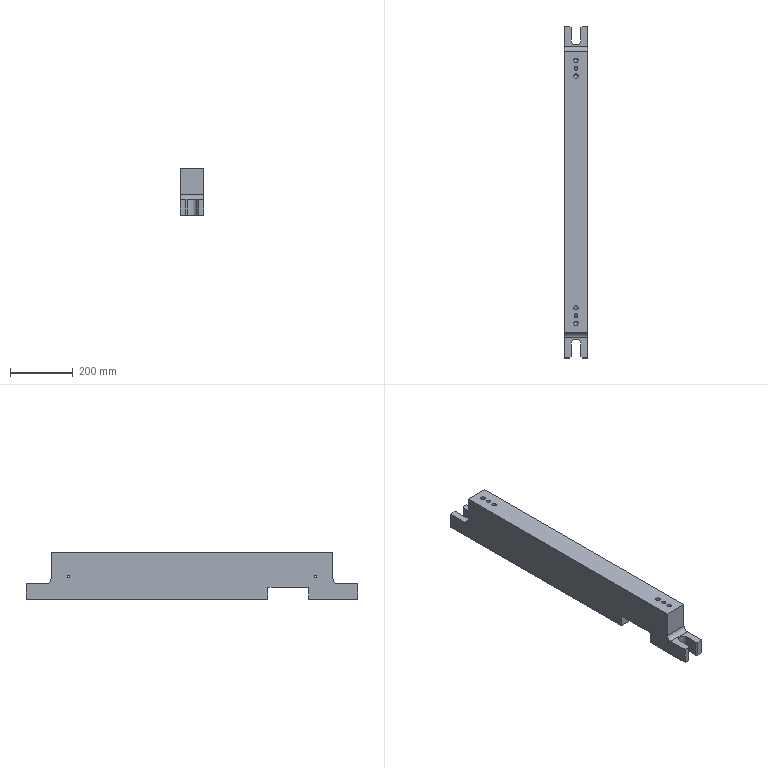Part | STEP file | 1_id734_x_t | 1 solid | 52 faces | box 75 x 1060 x 149.325 mm | volume 10048750 mm3 | plane 26 | cylinder 16 | cone 10 | commonest cylinder face diameters 12.7 x4 14 x4 8 x2 10.716 x2 30 x2 31.75 x2